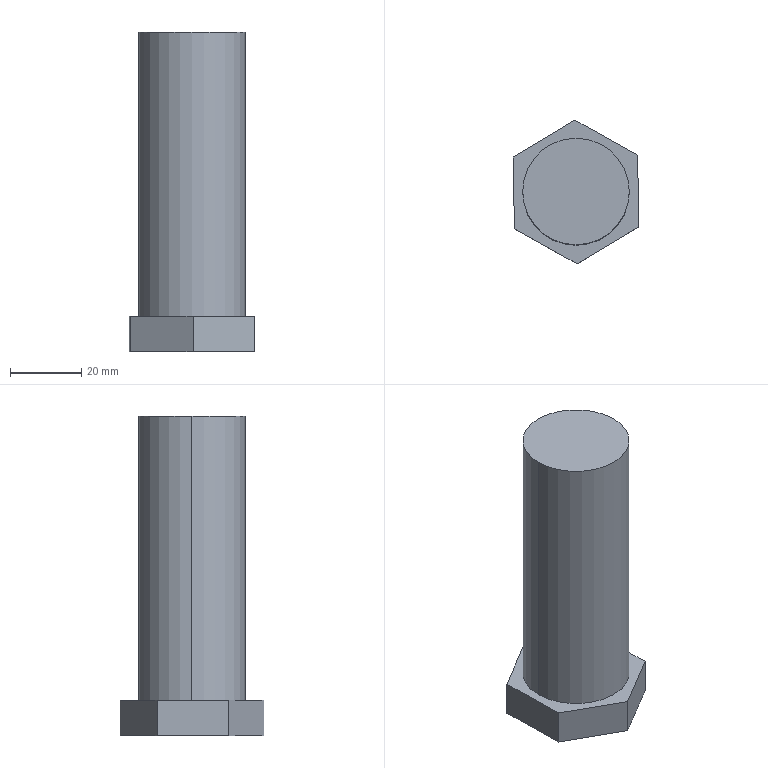Part | SolidWorks | features Extrusion 1, ICE 1 | 1 solid | 11 faces | box 35.299 x 40.41 x 90 mm | volume 67157 mm3 | plane 9 | cylinder 2 | commonest cylinder face diameters 30 x2
STEP:
#1=CARTESIAN_POINT('',(15.,0.,90.));
#2=VERTEX_POINT('',#1);
#3=CARTESIAN_POINT('',(-15.,0.,90.));
#4=VERTEX_POINT('',#3);
#5=CARTESIAN_POINT('',(0.,0.,90.));
#6=DIRECTION('',(0.,0.,1.));
#7=DIRECTION('',(1.,0.,0.));
#8=AXIS2_PLACEMENT_3D('',#5,#6,#7);
#9=CIRCLE('',#8,15.);
#10=EDGE_CURVE('',#2,#4,#9,.T.);
#11=ORIENTED_EDGE('',*,*,#10,.F.);
#12=CARTESIAN_POINT('',(15.,0.,10.));
#13=VERTEX_POINT('',#12);
#14=CARTESIAN_POINT('',(15.,0.,90.));
#15=DIRECTION('',(0.,0.,-1.));
#16=VECTOR('',#15,1000.);
#17=LINE('',#14,#16);
#18=EDGE_CURVE('',#2,#13,#17,.T.);
#19=ORIENTED_EDGE('',*,*,#18,.T.);
#20=CARTESIAN_POINT('',(-15.,0.,10.));
#21=VERTEX_POINT('',#20);
#22=CARTESIAN_POINT('',(0.,0.,10.));
#23=DIRECTION('',(0.,0.,1.));
#24=DIRECTION('',(1.,0.,0.));
#25=AXIS2_PLACEMENT_3D('',#22,#23,#24);
#26=CIRCLE('',#25,15.);
#27=EDGE_CURVE('',#13,#21,#26,.T.);
#28=ORIENTED_EDGE('',*,*,#27,.T.);
#29=CARTESIAN_POINT('',(-15.,0.,90.));
#30=DIRECTION('',(0.,0.,-1.));
#31=VECTOR('',#30,1000.);
#32=LINE('',#29,#31);
#33=EDGE_CURVE('',#4,#21,#32,.T.);
#34=ORIENTED_EDGE('',*,*,#33,.F.);
#35=EDGE_LOOP('',(#11,#19,#28,#34));
#36=FACE_OUTER_BOUND('',#35,.T.);
#37=CARTESIAN_POINT('',(0.,0.,90.));
#38=DIRECTION('',(0.,0.,-1.));
#39=DIRECTION('',(-1.,0.,0.));
#40=AXIS2_PLACEMENT_3D('',#37,#38,#39);
#41=CYLINDRICAL_SURFACE('',#40,15.);
#42=ADVANCED_FACE('',(#36),#41,.T.);
#43=CARTESIAN_POINT('',(17.65,-9.84,0.));
#44=VERTEX_POINT('',#43);
#45=CARTESIAN_POINT('',(17.347,10.365,0.));
#46=VERTEX_POINT('',#45);
#47=CARTESIAN_POINT('',(17.65,-9.84,0.));
#48=DIRECTION('',(-0.015,0.9999,0.));
#49=VECTOR('',#48,1000.);
#50=LINE('',#47,#49);
#51=EDGE_CURVE('',#44,#46,#50,.T.);
#52=ORIENTED_EDGE('',*,*,#51,.T.);
#53=CARTESIAN_POINT('',(17.347,10.365,10.));
#54=VERTEX_POINT('',#53);
#55=CARTESIAN_POINT('',(17.347,10.365,10.));
#56=DIRECTION('',(0.,0.,-1.));
#57=VECTOR('',#56,1000.);
#58=LINE('',#55,#57);
#59=EDGE_CURVE('',#54,#46,#58,.T.);
#60=ORIENTED_EDGE('',*,*,#59,.F.);
#61=CARTESIAN_POINT('',(17.65,-9.84,10.));
#62=VERTEX_POINT('',#61);
#63=CARTESIAN_POINT('',(17.65,-9.84,10.));
#64=DIRECTION('',(-0.015,0.9999,0.));
#65=VECTOR('',#64,1000.);
#66=LINE('',#63,#65);
#67=EDGE_CURVE('',#62,#54,#66,.T.);
#68=ORIENTED_EDGE('',*,*,#67,.F.);
#69=CARTESIAN_POINT('',(17.65,-9.84,10.));
#70=DIRECTION('',(0.,0.,-1.));
#71=VECTOR('',#70,1000.);
#72=LINE('',#69,#71);
#73=EDGE_CURVE('',#62,#44,#72,.T.);
#74=ORIENTED_EDGE('',*,*,#73,.T.);
#75=EDGE_LOOP('',(#52,#60,#68,#74));
#76=FACE_OUTER_BOUND('',#75,.T.);
#77=CARTESIAN_POINT('',(17.65,-9.84,10.));
#78=DIRECTION('',(-0.9999,-0.015,0.));
#79=DIRECTION('',(0.015,-0.9999,0.));
#80=AXIS2_PLACEMENT_3D('',#77,#78,#79);
#81=PLANE('',#80);
#82=ADVANCED_FACE('',(#76),#81,.F.);
#83=CARTESIAN_POINT('',(-0.303,20.205,0.));
#84=VERTEX_POINT('',#83);
#85=CARTESIAN_POINT('',(17.347,10.365,0.));
#86=DIRECTION('',(-0.8734,0.487,0.));
#87=VECTOR('',#86,1000.);
#88=LINE('',#85,#87);
#89=EDGE_CURVE('',#46,#84,#88,.T.);
#90=ORIENTED_EDGE('',*,*,#89,.T.);
#91=CARTESIAN_POINT('',(-0.303,20.205,10.));
#92=VERTEX_POINT('',#91);
#93=CARTESIAN_POINT('',(-0.303,20.205,10.));
#94=DIRECTION('',(0.,0.,-1.));
#95=VECTOR('',#94,1000.);
#96=LINE('',#93,#95);
#97=EDGE_CURVE('',#92,#84,#96,.T.);
#98=ORIENTED_EDGE('',*,*,#97,.F.);
#99=CARTESIAN_POINT('',(17.347,10.365,10.));
#100=DIRECTION('',(-0.8734,0.487,0.));
#101=VECTOR('',#100,1000.);
#102=LINE('',#99,#101);
#103=EDGE_CURVE('',#54,#92,#102,.T.);
#104=ORIENTED_EDGE('',*,*,#103,.F.);
#105=ORIENTED_EDGE('',*,*,#59,.T.);
#106=EDGE_LOOP('',(#90,#98,#104,#105));
#107=FACE_OUTER_BOUND('',#106,.T.);
#108=CARTESIAN_POINT('',(17.347,10.365,10.));
#109=DIRECTION('',(-0.487,-0.8734,0.));
#110=DIRECTION('',(0.8734,-0.487,0.));
#111=AXIS2_PLACEMENT_3D('',#108,#109,#110);
#112=PLANE('',#111);
#113=ADVANCED_FACE('',(#107),#112,.F.);
#114=CARTESIAN_POINT('',(-17.65,9.84,0.));
#115=VERTEX_POINT('',#114);
#116=CARTESIAN_POINT('',(-0.303,20.205,0.));
#117=DIRECTION('',(-0.8584,-0.5129,0.));
#118=VECTOR('',#117,1000.);
#119=LINE('',#116,#118);
#120=EDGE_CURVE('',#84,#115,#119,.T.);
#121=ORIENTED_EDGE('',*,*,#120,.T.);
#122=CARTESIAN_POINT('',(-17.65,9.84,10.));
#123=VERTEX_POINT('',#122);
#124=CARTESIAN_POINT('',(-17.65,9.84,10.));
#125=DIRECTION('',(0.,0.,-1.));
#126=VECTOR('',#125,1000.);
#127=LINE('',#124,#126);
#128=EDGE_CURVE('',#123,#115,#127,.T.);
#129=ORIENTED_EDGE('',*,*,#128,.F.);
#130=CARTESIAN_POINT('',(-0.303,20.205,10.));
#131=DIRECTION('',(-0.8584,-0.5129,0.));
#132=VECTOR('',#131,1000.);
#133=LINE('',#130,#132);
#134=EDGE_CURVE('',#92,#123,#133,.T.);
#135=ORIENTED_EDGE('',*,*,#134,.F.);
#136=ORIENTED_EDGE('',*,*,#97,.T.);
#137=EDGE_LOOP('',(#121,#129,#135,#136));
#138=FACE_OUTER_BOUND('',#137,.T.);
#139=CARTESIAN_POINT('',(-0.303,20.205,10.));
#140=DIRECTION('',(0.5129,-0.8584,0.));
#141=DIRECTION('',(0.8584,0.5129,0.));
#142=AXIS2_PLACEMENT_3D('',#139,#140,#141);
#143=PLANE('',#142);
#144=ADVANCED_FACE('',(#138),#143,.F.);
#145=CARTESIAN_POINT('',(-17.347,-10.365,0.));
#146=VERTEX_POINT('',#145);
#147=CARTESIAN_POINT('',(-17.65,9.84,0.));
#148=DIRECTION('',(0.015,-0.9999,0.));
#149=VECTOR('',#148,1000.);
#150=LINE('',#147,#149);
#151=EDGE_CURVE('',#115,#146,#150,.T.);
#152=ORIENTED_EDGE('',*,*,#151,.T.);
#153=CARTESIAN_POINT('',(-17.347,-10.365,10.));
#154=VERTEX_POINT('',#153);
#155=CARTESIAN_POINT('',(-17.347,-10.365,10.));
#156=DIRECTION('',(0.,0.,-1.));
#157=VECTOR('',#156,1000.);
#158=LINE('',#155,#157);
#159=EDGE_CURVE('',#154,#146,#158,.T.);
#160=ORIENTED_EDGE('',*,*,#159,.F.);
#161=CARTESIAN_POINT('',(-17.65,9.84,10.));
#162=DIRECTION('',(0.015,-0.9999,0.));
#163=VECTOR('',#162,1000.);
#164=LINE('',#161,#163);
#165=EDGE_CURVE('',#123,#154,#164,.T.);
#166=ORIENTED_EDGE('',*,*,#165,.F.);
#167=ORIENTED_EDGE('',*,*,#128,.T.);
#168=EDGE_LOOP('',(#152,#160,#166,#167));
#169=FACE_OUTER_BOUND('',#168,.T.);
#170=CARTESIAN_POINT('',(-17.65,9.84,10.));
#171=DIRECTION('',(0.9999,0.015,0.));
#172=DIRECTION('',(-0.015,0.9999,0.));
#173=AXIS2_PLACEMENT_3D('',#170,#171,#172);
#174=PLANE('',#173);
#175=ADVANCED_FACE('',(#169),#174,.F.);
#176=CARTESIAN_POINT('',(0.303,-20.205,0.));
#177=VERTEX_POINT('',#176);
#178=CARTESIAN_POINT('',(-17.347,-10.365,0.));
#179=DIRECTION('',(0.8734,-0.487,0.));
#180=VECTOR('',#179,1000.);
#181=LINE('',#178,#180);
#182=EDGE_CURVE('',#146,#177,#181,.T.);
#183=ORIENTED_EDGE('',*,*,#182,.T.);
#184=CARTESIAN_POINT('',(0.303,-20.205,10.));
#185=VERTEX_POINT('',#184);
#186=CARTESIAN_POINT('',(0.303,-20.205,10.));
#187=DIRECTION('',(0.,0.,-1.));
#188=VECTOR('',#187,1000.);
#189=LINE('',#186,#188);
#190=EDGE_CURVE('',#185,#177,#189,.T.);
#191=ORIENTED_EDGE('',*,*,#190,.F.);
#192=CARTESIAN_POINT('',(-17.347,-10.365,10.));
#193=DIRECTION('',(0.8734,-0.487,0.));
#194=VECTOR('',#193,1000.);
#195=LINE('',#192,#194);
#196=EDGE_CURVE('',#154,#185,#195,.T.);
#197=ORIENTED_EDGE('',*,*,#196,.F.);
#198=ORIENTED_EDGE('',*,*,#159,.T.);
#199=EDGE_LOOP('',(#183,#191,#197,#198));
#200=FACE_OUTER_BOUND('',#199,.T.);
#201=CARTESIAN_POINT('',(-17.347,-10.365,10.));
#202=DIRECTION('',(0.487,0.8734,0.));
#203=DIRECTION('',(-0.8734,0.487,0.));
#204=AXIS2_PLACEMENT_3D('',#201,#202,#203);
#205=PLANE('',#204);
#206=ADVANCED_FACE('',(#200),#205,.F.);
#207=CARTESIAN_POINT('',(0.303,-20.205,0.));
#208=DIRECTION('',(0.8584,0.5129,0.));
#209=VECTOR('',#208,1000.);
#210=LINE('',#207,#209);
#211=EDGE_CURVE('',#177,#44,#210,.T.);
#212=ORIENTED_EDGE('',*,*,#211,.T.);
#213=ORIENTED_EDGE('',*,*,#73,.F.);
#214=CARTESIAN_POINT('',(0.303,-20.205,10.));
#215=DIRECTION('',(0.8584,0.5129,0.));
#216=VECTOR('',#215,1000.);
#217=LINE('',#214,#216);
#218=EDGE_CURVE('',#185,#62,#217,.T.);
#219=ORIENTED_EDGE('',*,*,#218,.F.);
#220=ORIENTED_EDGE('',*,*,#190,.T.);
#221=EDGE_LOOP('',(#212,#213,#219,#220));
#222=FACE_OUTER_BOUND('',#221,.T.);
#223=CARTESIAN_POINT('',(0.303,-20.205,10.));
#224=DIRECTION('',(-0.5129,0.8584,0.));
#225=DIRECTION('',(-0.8584,-0.5129,0.));
#226=AXIS2_PLACEMENT_3D('',#223,#224,#225);
#227=PLANE('',#226);
#228=ADVANCED_FACE('',(#222),#227,.F.);
#229=CARTESIAN_POINT('',(0.,0.,10.));
#230=DIRECTION('',(0.,0.,1.));
#231=DIRECTION('',(1.,0.,0.));
#232=AXIS2_PLACEMENT_3D('',#229,#230,#231);
#233=CIRCLE('',#232,15.);
#234=EDGE_CURVE('',#21,#13,#233,.T.);
#235=ORIENTED_EDGE('',*,*,#234,.F.);
#236=ORIENTED_EDGE('',*,*,#27,.F.);
#237=EDGE_LOOP('',(#235,#236));
#238=FACE_BOUND('',#237,.T.);
#239=ORIENTED_EDGE('',*,*,#67,.T.);
#240=ORIENTED_EDGE('',*,*,#103,.T.);
#241=ORIENTED_EDGE('',*,*,#134,.T.);
#242=ORIENTED_EDGE('',*,*,#165,.T.);
#243=ORIENTED_EDGE('',*,*,#196,.T.);
#244=ORIENTED_EDGE('',*,*,#218,.T.);
#245=EDGE_LOOP('',(#239,#240,#241,#242,#243,#244));
#246=FACE_OUTER_BOUND('',#245,.T.);
#247=CARTESIAN_POINT('',(0.,0.,10.));
#248=DIRECTION('',(0.,0.,1.));
#249=DIRECTION('',(1.,0.,0.));
#250=AXIS2_PLACEMENT_3D('',#247,#248,#249);
#251=PLANE('',#250);
#252=ADVANCED_FACE('',(#238,#246),#251,.T.);
#253=ORIENTED_EDGE('',*,*,#51,.F.);
#254=ORIENTED_EDGE('',*,*,#211,.F.);
#255=ORIENTED_EDGE('',*,*,#182,.F.);
#256=ORIENTED_EDGE('',*,*,#151,.F.);
#257=ORIENTED_EDGE('',*,*,#120,.F.);
#258=ORIENTED_EDGE('',*,*,#89,.F.);
#259=EDGE_LOOP('',(#253,#254,#255,#256,#257,#258));
#260=FACE_OUTER_BOUND('',#259,.T.);
#261=CARTESIAN_POINT('',(0.,0.,0.));
#262=DIRECTION('',(0.,0.,1.));
#263=DIRECTION('',(1.,0.,0.));
#264=AXIS2_PLACEMENT_3D('',#261,#262,#263);
#265=PLANE('',#264);
#266=ADVANCED_FACE('',(#260),#265,.F.);
#267=ORIENTED_EDGE('',*,*,#18,.F.);
#268=CARTESIAN_POINT('',(0.,0.,90.));
#269=DIRECTION('',(0.,0.,1.));
#270=DIRECTION('',(1.,0.,0.));
#271=AXIS2_PLACEMENT_3D('',#268,#269,#270);
#272=CIRCLE('',#271,15.);
#273=EDGE_CURVE('',#4,#2,#272,.T.);
#274=ORIENTED_EDGE('',*,*,#273,.F.);
#275=ORIENTED_EDGE('',*,*,#33,.T.);
#276=ORIENTED_EDGE('',*,*,#234,.T.);
#277=EDGE_LOOP('',(#267,#274,#275,#276));
#278=FACE_OUTER_BOUND('',#277,.T.);
#279=CARTESIAN_POINT('',(0.,0.,90.));
#280=DIRECTION('',(0.,0.,-1.));
#281=DIRECTION('',(-1.,0.,0.));
#282=AXIS2_PLACEMENT_3D('',#279,#280,#281);
#283=CYLINDRICAL_SURFACE('',#282,15.);
#284=ADVANCED_FACE('',(#278),#283,.T.);
#285=ORIENTED_EDGE('',*,*,#273,.T.);
#286=ORIENTED_EDGE('',*,*,#10,.T.);
#287=EDGE_LOOP('',(#285,#286));
#288=FACE_OUTER_BOUND('',#287,.T.);
#289=CARTESIAN_POINT('',(0.,0.,90.));
#290=DIRECTION('',(0.,0.,1.));
#291=DIRECTION('',(1.,0.,0.));
#292=AXIS2_PLACEMENT_3D('',#289,#290,#291);
#293=PLANE('',#292);
#294=ADVANCED_FACE('',(#288),#293,.T.);
#295=CLOSED_SHELL('',(#42,#82,#113,#144,#175,#206,#228,#252,#266,#284,#294));
#296=MANIFOLD_SOLID_BREP('',#295);
#297=CARTESIAN_POINT('',(0.,0.,0.));
#298=DIRECTION('',(0.,0.,1.));
#299=DIRECTION('',(1.,0.,0.));
#300=AXIS2_PLACEMENT_3D('',#297,#298,#299);
#301=(LENGTH_UNIT()NAMED_UNIT(*)SI_UNIT(.MILLI.,.METRE.));
#302=UNCERTAINTY_MEASURE_WITH_UNIT(LENGTH_MEASURE(0.00001),#301,'','');
#303=(NAMED_UNIT(*)PLANE_ANGLE_UNIT()SI_UNIT($,.RADIAN.));
#304=(NAMED_UNIT(*)SI_UNIT($,.STERADIAN.)SOLID_ANGLE_UNIT());
#305=(GEOMETRIC_REPRESENTATION_CONTEXT(3)GLOBAL_UNCERTAINTY_ASSIGNED_CONTEXT((#302))GLOBAL_UNIT_ASSIGNED_CONTEXT((#301,#303,#304))REPRESENTATION_CONTEXT('',''));
#306=ADVANCED_BREP_SHAPE_REPRESENTATION('',(#296,#300),#305);